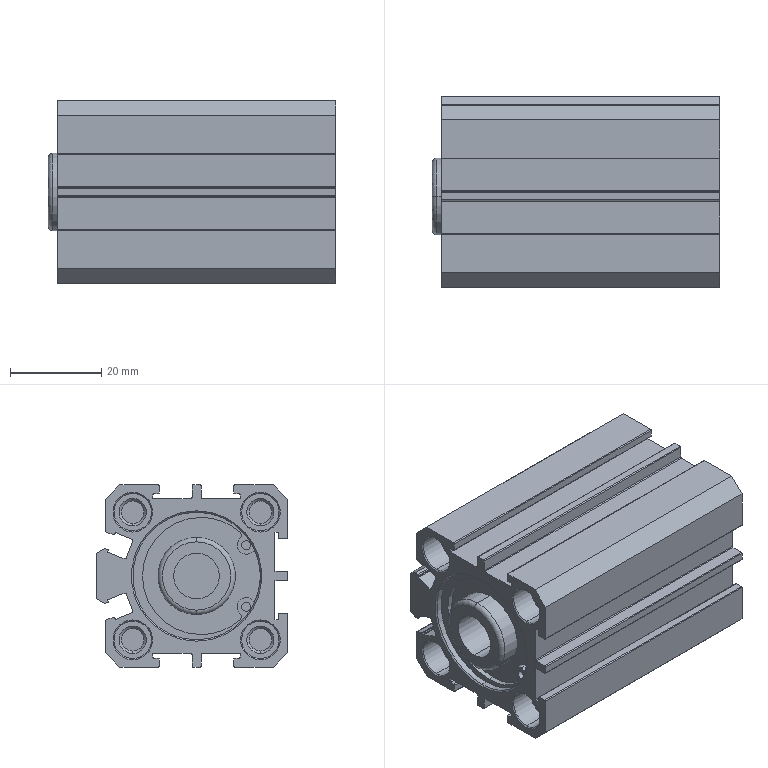Part | SolidWorks | features RefAxis 21, 3DProfileFeature 7, RevCut 6, Extrusion 1, ICE 1, LPattern 1, Revolution 1 | 1 solid | 232 faces | box 63 x 42 x 40 mm | volume 56645 mm3 | cylinder 103 | plane 87 | cone 40 | torus 2 | commonest cylinder face diameters 0.4 x46 8.2 x16 4.917 x8 0.8 x7 2 x6 4.134 x4